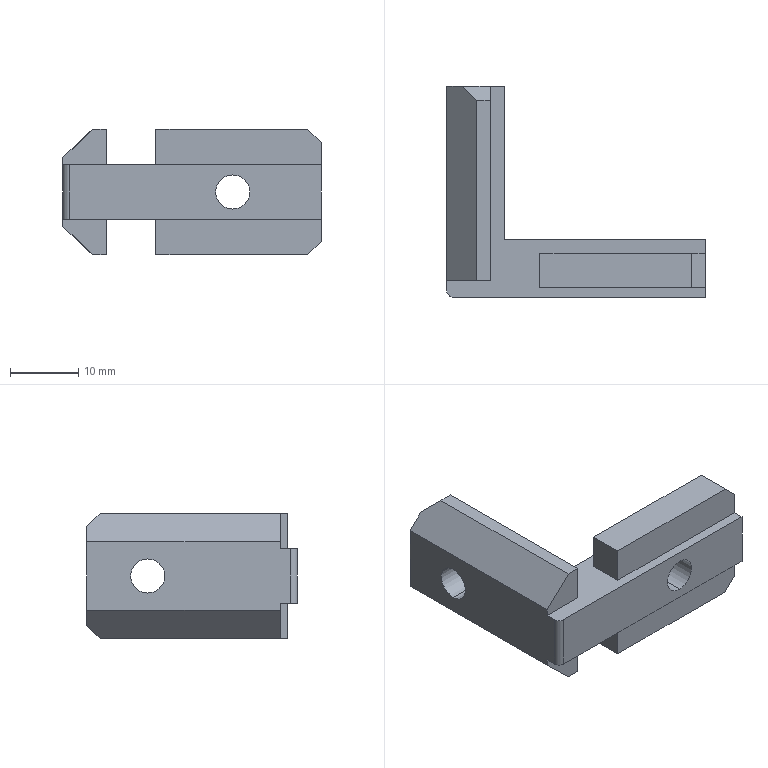Part | STEP file | New in-slot right-angle connector, 40 series (with set screw) | 1 solid | 33 faces | box 38 x 31 x 18.5 mm | volume 6406 mm3 | plane 28 | cylinder 5 | commonest cylinder face diameters 5 x4 2 x1